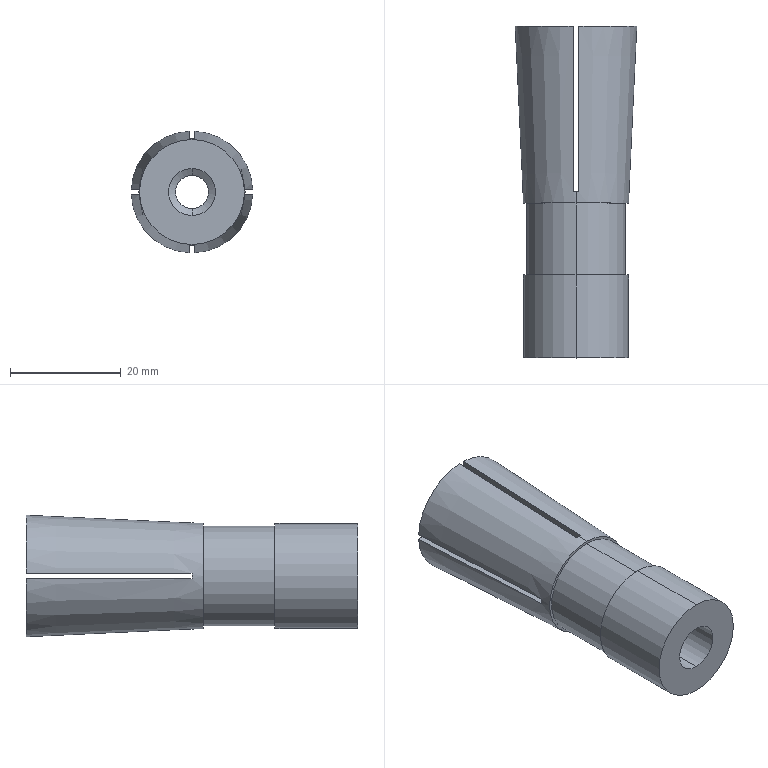Part | SolidWorks | features ICE 3, 3DProfileFeature 1, HoleWzd 1, Revolution 1 | 1 solid | 31 faces | box 21.977 x 60 x 21.977 mm | volume 14861 mm3 | plane 19 | cylinder 8 | cone 4 | commonest cylinder face diameters 6 x2 8.5 x2 18 x2 19 x2
STEP:
#1=CARTESIAN_POINT('',(0.,24.5,4.25));
#2=VERTEX_POINT('',#1);
#3=CARTESIAN_POINT('',(0.,24.5,-4.25));
#4=VERTEX_POINT('',#3);
#5=CARTESIAN_POINT('',(0.,24.5,0.));
#6=DIRECTION('',(0.,-1.,0.));
#7=DIRECTION('',(0.,0.,-1.));
#8=AXIS2_PLACEMENT_3D('',#5,#6,#7);
#9=CIRCLE('',#8,4.25);
#10=EDGE_CURVE('',#2,#4,#9,.T.);
#11=ORIENTED_EDGE('',*,*,#10,.F.);
#12=CARTESIAN_POINT('',(0.,0.,4.25));
#13=VERTEX_POINT('',#12);
#14=CARTESIAN_POINT('',(0.,0.,4.25));
#15=DIRECTION('',(0.,-1.,0.));
#16=VECTOR('',#15,1000.);
#17=LINE('',#14,#16);
#18=EDGE_CURVE('',#2,#13,#17,.T.);
#19=ORIENTED_EDGE('',*,*,#18,.T.);
#20=CARTESIAN_POINT('',(0.,0.,-4.25));
#21=VERTEX_POINT('',#20);
#22=CARTESIAN_POINT('',(0.,0.,0.));
#23=DIRECTION('',(0.,-1.,0.));
#24=DIRECTION('',(0.,0.,-1.));
#25=AXIS2_PLACEMENT_3D('',#22,#23,#24);
#26=CIRCLE('',#25,4.25);
#27=EDGE_CURVE('',#13,#21,#26,.T.);
#28=ORIENTED_EDGE('',*,*,#27,.T.);
#29=CARTESIAN_POINT('',(0.,0.,-4.25));
#30=DIRECTION('',(0.,-1.,0.));
#31=VECTOR('',#30,1000.);
#32=LINE('',#29,#31);
#33=EDGE_CURVE('',#4,#21,#32,.T.);
#34=ORIENTED_EDGE('',*,*,#33,.F.);
#35=EDGE_LOOP('',(#11,#19,#28,#34));
#36=FACE_OUTER_BOUND('',#35,.T.);
#37=CARTESIAN_POINT('',(0.,0.,0.));
#38=DIRECTION('',(0.,-1.,0.));
#39=DIRECTION('',(0.,0.,-1.));
#40=AXIS2_PLACEMENT_3D('',#37,#38,#39);
#41=CYLINDRICAL_SURFACE('',#40,4.25);
#42=ADVANCED_FACE('',(#36),#41,.F.);
#43=CARTESIAN_POINT('',(0.,25.251,3.));
#44=VERTEX_POINT('',#43);
#45=CARTESIAN_POINT('',(0.,25.251,-3.));
#46=VERTEX_POINT('',#45);
#47=CARTESIAN_POINT('',(0.,25.251,0.));
#48=DIRECTION('',(0.,-1.,0.));
#49=DIRECTION('',(0.,0.,-1.));
#50=AXIS2_PLACEMENT_3D('',#47,#48,#49);
#51=CIRCLE('',#50,3.);
#52=EDGE_CURVE('',#44,#46,#51,.T.);
#53=ORIENTED_EDGE('',*,*,#52,.F.);
#54=CARTESIAN_POINT('',(0.,24.5,4.25));
#55=DIRECTION('',(0.,-0.515,0.8572));
#56=VECTOR('',#55,1000.);
#57=LINE('',#54,#56);
#58=EDGE_CURVE('',#44,#2,#57,.T.);
#59=ORIENTED_EDGE('',*,*,#58,.T.);
#60=ORIENTED_EDGE('',*,*,#10,.T.);
#61=CARTESIAN_POINT('',(0.,24.5,-4.25));
#62=DIRECTION('',(0.,-0.515,-0.8572));
#63=VECTOR('',#62,1000.);
#64=LINE('',#61,#63);
#65=EDGE_CURVE('',#46,#4,#64,.T.);
#66=ORIENTED_EDGE('',*,*,#65,.F.);
#67=EDGE_LOOP('',(#53,#59,#60,#66));
#68=FACE_OUTER_BOUND('',#67,.T.);
#69=CARTESIAN_POINT('',(0.,24.5,0.));
#70=DIRECTION('',(0.,-1.,0.));
#71=DIRECTION('',(0.,0.,-1.));
#72=AXIS2_PLACEMENT_3D('',#69,#70,#71);
#73=CONICAL_SURFACE('',#72,4.25,1.03);
#74=ADVANCED_FACE('',(#68),#73,.F.);
#75=ORIENTED_EDGE('',*,*,#52,.T.);
#76=CARTESIAN_POINT('',(0.,30.,-3.));
#77=VERTEX_POINT('',#76);
#78=CARTESIAN_POINT('',(0.,0.,-3.));
#79=DIRECTION('',(0.,1.,0.));
#80=VECTOR('',#79,1000.);
#81=LINE('',#78,#80);
#82=EDGE_CURVE('',#46,#77,#81,.T.);
#83=ORIENTED_EDGE('',*,*,#82,.T.);
#84=CARTESIAN_POINT('',(-0.5,30.,-2.958));
#85=VERTEX_POINT('',#84);
#86=CARTESIAN_POINT('',(0.,30.,0.));
#87=DIRECTION('',(0.,1.,0.));
#88=DIRECTION('',(0.,0.,-1.));
#89=AXIS2_PLACEMENT_3D('',#86,#87,#88);
#90=CIRCLE('',#89,3.);
#91=EDGE_CURVE('',#77,#85,#90,.T.);
#92=ORIENTED_EDGE('',*,*,#91,.T.);
#93=CARTESIAN_POINT('',(-0.5,60.,-2.958));
#94=VERTEX_POINT('',#93);
#95=CARTESIAN_POINT('',(-0.5,0.,-2.958));
#96=DIRECTION('',(0.,1.,0.));
#97=VECTOR('',#96,1000.);
#98=LINE('',#95,#97);
#99=EDGE_CURVE('',#85,#94,#98,.T.);
#100=ORIENTED_EDGE('',*,*,#99,.T.);
#101=CARTESIAN_POINT('',(-2.958,60.,-0.5));
#102=VERTEX_POINT('',#101);
#103=CARTESIAN_POINT('',(0.,60.,0.));
#104=DIRECTION('',(0.,1.,0.));
#105=DIRECTION('',(0.,0.,1.));
#106=AXIS2_PLACEMENT_3D('',#103,#104,#105);
#107=CIRCLE('',#106,3.);
#108=EDGE_CURVE('',#94,#102,#107,.T.);
#109=ORIENTED_EDGE('',*,*,#108,.T.);
#110=CARTESIAN_POINT('',(-2.958,30.,-0.5));
#111=VERTEX_POINT('',#110);
#112=CARTESIAN_POINT('',(-2.958,0.,-0.5));
#113=DIRECTION('',(0.,-1.,0.));
#114=VECTOR('',#113,1000.);
#115=LINE('',#112,#114);
#116=EDGE_CURVE('',#102,#111,#115,.T.);
#117=ORIENTED_EDGE('',*,*,#116,.T.);
#118=CARTESIAN_POINT('',(-2.958,30.,0.5));
#119=VERTEX_POINT('',#118);
#120=CARTESIAN_POINT('',(0.,30.,0.));
#121=DIRECTION('',(0.,-1.,0.));
#122=DIRECTION('',(0.,0.,1.));
#123=AXIS2_PLACEMENT_3D('',#120,#121,#122);
#124=CIRCLE('',#123,3.);
#125=EDGE_CURVE('',#119,#111,#124,.T.);
#126=ORIENTED_EDGE('',*,*,#125,.F.);
#127=CARTESIAN_POINT('',(-2.958,60.,0.5));
#128=VERTEX_POINT('',#127);
#129=CARTESIAN_POINT('',(-2.958,0.,0.5));
#130=DIRECTION('',(0.,1.,0.));
#131=VECTOR('',#130,1000.);
#132=LINE('',#129,#131);
#133=EDGE_CURVE('',#119,#128,#132,.T.);
#134=ORIENTED_EDGE('',*,*,#133,.T.);
#135=CARTESIAN_POINT('',(-0.5,60.,2.958));
#136=VERTEX_POINT('',#135);
#137=CARTESIAN_POINT('',(0.,60.,0.));
#138=DIRECTION('',(0.,1.,0.));
#139=DIRECTION('',(0.,0.,1.));
#140=AXIS2_PLACEMENT_3D('',#137,#138,#139);
#141=CIRCLE('',#140,3.);
#142=EDGE_CURVE('',#128,#136,#141,.T.);
#143=ORIENTED_EDGE('',*,*,#142,.T.);
#144=CARTESIAN_POINT('',(-0.5,30.,2.958));
#145=VERTEX_POINT('',#144);
#146=CARTESIAN_POINT('',(-0.5,0.,2.958));
#147=DIRECTION('',(0.,-1.,0.));
#148=VECTOR('',#147,1000.);
#149=LINE('',#146,#148);
#150=EDGE_CURVE('',#136,#145,#149,.T.);
#151=ORIENTED_EDGE('',*,*,#150,.T.);
#152=CARTESIAN_POINT('',(0.,30.,3.));
#153=VERTEX_POINT('',#152);
#154=CARTESIAN_POINT('',(0.,30.,0.));
#155=DIRECTION('',(0.,1.,0.));
#156=DIRECTION('',(0.,0.,-1.));
#157=AXIS2_PLACEMENT_3D('',#154,#155,#156);
#158=CIRCLE('',#157,3.);
#159=EDGE_CURVE('',#145,#153,#158,.T.);
#160=ORIENTED_EDGE('',*,*,#159,.T.);
#161=CARTESIAN_POINT('',(0.,0.,3.));
#162=DIRECTION('',(0.,1.,0.));
#163=VECTOR('',#162,1000.);
#164=LINE('',#161,#163);
#165=EDGE_CURVE('',#44,#153,#164,.T.);
#166=ORIENTED_EDGE('',*,*,#165,.F.);
#167=EDGE_LOOP('',(#75,#83,#92,#100,#109,#117,#126,#134,#143,#151,#160,#166));
#168=FACE_OUTER_BOUND('',#167,.T.);
#169=CARTESIAN_POINT('',(0.,0.,0.));
#170=DIRECTION('',(0.,1.,0.));
#171=DIRECTION('',(0.,0.,1.));
#172=AXIS2_PLACEMENT_3D('',#169,#170,#171);
#173=CYLINDRICAL_SURFACE('',#172,3.);
#174=ADVANCED_FACE('',(#168),#173,.F.);
#175=CARTESIAN_POINT('',(0.,15.,-9.5));
#176=VERTEX_POINT('',#175);
#177=CARTESIAN_POINT('',(0.,15.,9.5));
#178=VERTEX_POINT('',#177);
#179=CARTESIAN_POINT('',(0.,15.,0.));
#180=DIRECTION('',(0.,-1.,0.));
#181=DIRECTION('',(0.,0.,-1.));
#182=AXIS2_PLACEMENT_3D('',#179,#180,#181);
#183=CIRCLE('',#182,9.5);
#184=EDGE_CURVE('',#176,#178,#183,.T.);
#185=ORIENTED_EDGE('',*,*,#184,.T.);
#186=CARTESIAN_POINT('',(0.,0.,9.5));
#187=VERTEX_POINT('',#186);
#188=CARTESIAN_POINT('',(0.,0.,9.5));
#189=DIRECTION('',(0.,-1.,0.));
#190=VECTOR('',#189,1000.);
#191=LINE('',#188,#190);
#192=EDGE_CURVE('',#178,#187,#191,.T.);
#193=ORIENTED_EDGE('',*,*,#192,.T.);
#194=CARTESIAN_POINT('',(0.,0.,-9.5));
#195=VERTEX_POINT('',#194);
#196=CARTESIAN_POINT('',(0.,0.,0.));
#197=DIRECTION('',(0.,-1.,0.));
#198=DIRECTION('',(0.,0.,-1.));
#199=AXIS2_PLACEMENT_3D('',#196,#197,#198);
#200=CIRCLE('',#199,9.5);
#201=EDGE_CURVE('',#195,#187,#200,.T.);
#202=ORIENTED_EDGE('',*,*,#201,.F.);
#203=CARTESIAN_POINT('',(0.,0.,-9.5));
#204=DIRECTION('',(0.,-1.,0.));
#205=VECTOR('',#204,1000.);
#206=LINE('',#203,#205);
#207=EDGE_CURVE('',#176,#195,#206,.T.);
#208=ORIENTED_EDGE('',*,*,#207,.F.);
#209=EDGE_LOOP('',(#185,#193,#202,#208));
#210=FACE_OUTER_BOUND('',#209,.T.);
#211=CARTESIAN_POINT('',(0.,0.,0.));
#212=DIRECTION('',(0.,-1.,0.));
#213=DIRECTION('',(0.,0.,-1.));
#214=AXIS2_PLACEMENT_3D('',#211,#212,#213);
#215=CYLINDRICAL_SURFACE('',#214,9.5);
#216=ADVANCED_FACE('',(#210),#215,.T.);
#217=CARTESIAN_POINT('',(0.,28.,-9.));
#218=VERTEX_POINT('',#217);
#219=CARTESIAN_POINT('',(0.,28.,9.));
#220=VERTEX_POINT('',#219);
#221=CARTESIAN_POINT('',(0.,28.,0.));
#222=DIRECTION('',(0.,-1.,0.));
#223=DIRECTION('',(0.,0.,-1.));
#224=AXIS2_PLACEMENT_3D('',#221,#222,#223);
#225=CIRCLE('',#224,9.);
#226=EDGE_CURVE('',#218,#220,#225,.T.);
#227=ORIENTED_EDGE('',*,*,#226,.T.);
#228=CARTESIAN_POINT('',(0.,15.,9.));
#229=VERTEX_POINT('',#228);
#230=CARTESIAN_POINT('',(0.,0.,9.));
#231=DIRECTION('',(0.,-1.,0.));
#232=VECTOR('',#231,1000.);
#233=LINE('',#230,#232);
#234=EDGE_CURVE('',#220,#229,#233,.T.);
#235=ORIENTED_EDGE('',*,*,#234,.T.);
#236=CARTESIAN_POINT('',(0.,15.,-9.));
#237=VERTEX_POINT('',#236);
#238=CARTESIAN_POINT('',(0.,15.,0.));
#239=DIRECTION('',(0.,-1.,0.));
#240=DIRECTION('',(0.,0.,-1.));
#241=AXIS2_PLACEMENT_3D('',#238,#239,#240);
#242=CIRCLE('',#241,9.);
#243=EDGE_CURVE('',#237,#229,#242,.T.);
#244=ORIENTED_EDGE('',*,*,#243,.F.);
#245=CARTESIAN_POINT('',(0.,0.,-9.));
#246=DIRECTION('',(0.,-1.,0.));
#247=VECTOR('',#246,1000.);
#248=LINE('',#245,#247);
#249=EDGE_CURVE('',#218,#237,#248,.T.);
#250=ORIENTED_EDGE('',*,*,#249,.F.);
#251=EDGE_LOOP('',(#227,#235,#244,#250));
#252=FACE_OUTER_BOUND('',#251,.T.);
#253=CARTESIAN_POINT('',(0.,0.,0.));
#254=DIRECTION('',(0.,-1.,0.));
#255=DIRECTION('',(0.,0.,-1.));
#256=AXIS2_PLACEMENT_3D('',#253,#254,#255);
#257=CYLINDRICAL_SURFACE('',#256,9.);
#258=ADVANCED_FACE('',(#252),#257,.T.);
#259=CARTESIAN_POINT('',(0.,28.,-9.5));
#260=VERTEX_POINT('',#259);
#261=CARTESIAN_POINT('',(0.,28.,9.5));
#262=VERTEX_POINT('',#261);
#263=CARTESIAN_POINT('',(0.,28.,0.));
#264=DIRECTION('',(0.,-1.,0.));
#265=DIRECTION('',(0.,0.,-1.));
#266=AXIS2_PLACEMENT_3D('',#263,#264,#265);
#267=CIRCLE('',#266,9.5);
#268=EDGE_CURVE('',#260,#262,#267,.T.);
#269=ORIENTED_EDGE('',*,*,#268,.F.);
#270=CARTESIAN_POINT('',(0.,30.,-9.594));
#271=VERTEX_POINT('',#270);
#272=CARTESIAN_POINT('',(0.,28.,-9.5));
#273=DIRECTION('',(0.,0.9989,-0.04682));
#274=VECTOR('',#273,1000.);
#275=LINE('',#272,#274);
#276=EDGE_CURVE('',#260,#271,#275,.T.);
#277=ORIENTED_EDGE('',*,*,#276,.T.);
#278=CARTESIAN_POINT('',(0.5,30.,-9.581));
#279=VERTEX_POINT('',#278);
#280=CARTESIAN_POINT('',(0.,30.,0.));
#281=DIRECTION('',(0.,1.,0.));
#282=DIRECTION('',(0.,0.,-1.));
#283=AXIS2_PLACEMENT_3D('',#280,#281,#282);
#284=CIRCLE('',#283,9.594);
#285=EDGE_CURVE('',#279,#271,#284,.T.);
#286=ORIENTED_EDGE('',*,*,#285,.F.);
#287=CARTESIAN_POINT('',(0.5,60.,-10.989));
#288=VERTEX_POINT('',#287);
#289=CARTESIAN_POINT('',(0.5,60.,-10.989));
#290=CARTESIAN_POINT('',(0.5,50.,-10.519));
#291=CARTESIAN_POINT('',(0.5,40.,-10.05));
#292=CARTESIAN_POINT('',(0.5,30.,-9.581));
#293=B_SPLINE_CURVE_WITH_KNOTS('',3,(#289,#290,#291,#292),.UNSPECIFIED.,.F.,.F.,(4,4),(0.03724,0.06728),.UNSPECIFIED.);
#294=EDGE_CURVE('',#288,#279,#293,.T.);
#295=ORIENTED_EDGE('',*,*,#294,.F.);
#296=CARTESIAN_POINT('',(10.989,60.,-0.5));
#297=VERTEX_POINT('',#296);
#298=CARTESIAN_POINT('',(0.,60.,0.));
#299=DIRECTION('',(0.,-1.,0.));
#300=DIRECTION('',(0.,0.,-1.));
#301=AXIS2_PLACEMENT_3D('',#298,#299,#300);
#302=CIRCLE('',#301,11.);
#303=EDGE_CURVE('',#288,#297,#302,.T.);
#304=ORIENTED_EDGE('',*,*,#303,.T.);
#305=CARTESIAN_POINT('',(9.581,30.,-0.5));
#306=VERTEX_POINT('',#305);
#307=CARTESIAN_POINT('',(9.581,30.,-0.5));
#308=CARTESIAN_POINT('',(10.05,40.,-0.5));
#309=CARTESIAN_POINT('',(10.519,50.,-0.5));
#310=CARTESIAN_POINT('',(10.989,60.,-0.5));
#311=B_SPLINE_CURVE_WITH_KNOTS('',3,(#307,#308,#309,#310),.UNSPECIFIED.,.F.,.F.,(4,4),(0.03724,0.06728),.UNSPECIFIED.);
#312=EDGE_CURVE('',#306,#297,#311,.T.);
#313=ORIENTED_EDGE('',*,*,#312,.F.);
#314=CARTESIAN_POINT('',(9.581,30.,0.5));
#315=VERTEX_POINT('',#314);
#316=CARTESIAN_POINT('',(0.,30.,0.));
#317=DIRECTION('',(0.,-1.,0.));
#318=DIRECTION('',(0.,0.,1.));
#319=AXIS2_PLACEMENT_3D('',#316,#317,#318);
#320=CIRCLE('',#319,9.594);
#321=EDGE_CURVE('',#306,#315,#320,.T.);
#322=ORIENTED_EDGE('',*,*,#321,.T.);
#323=CARTESIAN_POINT('',(10.989,60.,0.5));
#324=VERTEX_POINT('',#323);
#325=CARTESIAN_POINT('',(10.989,60.,0.5));
#326=CARTESIAN_POINT('',(10.519,50.,0.5));
#327=CARTESIAN_POINT('',(10.05,40.,0.5));
#328=CARTESIAN_POINT('',(9.581,30.,0.5));
#329=B_SPLINE_CURVE_WITH_KNOTS('',3,(#325,#326,#327,#328),.UNSPECIFIED.,.F.,.F.,(4,4),(0.03724,0.06728),.UNSPECIFIED.);
#330=EDGE_CURVE('',#324,#315,#329,.T.);
#331=ORIENTED_EDGE('',*,*,#330,.F.);
#332=CARTESIAN_POINT('',(0.5,60.,10.989));
#333=VERTEX_POINT('',#332);
#334=CARTESIAN_POINT('',(0.,60.,0.));
#335=DIRECTION('',(0.,-1.,0.));
#336=DIRECTION('',(0.,0.,-1.));
#337=AXIS2_PLACEMENT_3D('',#334,#335,#336);
#338=CIRCLE('',#337,11.);
#339=EDGE_CURVE('',#324,#333,#338,.T.);
#340=ORIENTED_EDGE('',*,*,#339,.T.);
#341=CARTESIAN_POINT('',(0.5,30.,9.581));
#342=VERTEX_POINT('',#341);
#343=CARTESIAN_POINT('',(0.5,30.,9.581));
#344=CARTESIAN_POINT('',(0.5,40.,10.05));
#345=CARTESIAN_POINT('',(0.5,50.,10.519));
#346=CARTESIAN_POINT('',(0.5,60.,10.989));
#347=B_SPLINE_CURVE_WITH_KNOTS('',3,(#343,#344,#345,#346),.UNSPECIFIED.,.F.,.F.,(4,4),(0.03724,0.06728),.UNSPECIFIED.);
#348=EDGE_CURVE('',#342,#333,#347,.T.);
#349=ORIENTED_EDGE('',*,*,#348,.F.);
#350=CARTESIAN_POINT('',(0.,30.,9.594));
#351=VERTEX_POINT('',#350);
#352=CARTESIAN_POINT('',(0.,30.,0.));
#353=DIRECTION('',(0.,1.,0.));
#354=DIRECTION('',(0.,0.,-1.));
#355=AXIS2_PLACEMENT_3D('',#352,#353,#354);
#356=CIRCLE('',#355,9.594);
#357=EDGE_CURVE('',#351,#342,#356,.T.);
#358=ORIENTED_EDGE('',*,*,#357,.F.);
#359=CARTESIAN_POINT('',(0.,28.,9.5));
#360=DIRECTION('',(0.,0.9989,0.04682));
#361=VECTOR('',#360,1000.);
#362=LINE('',#359,#361);
#363=EDGE_CURVE('',#262,#351,#362,.T.);
#364=ORIENTED_EDGE('',*,*,#363,.F.);
#365=EDGE_LOOP('',(#269,#277,#286,#295,#304,#313,#322,#331,#340,#349,#358,#364));
#366=FACE_OUTER_BOUND('',#365,.T.);
#367=CARTESIAN_POINT('',(0.,28.,0.));
#368=DIRECTION('',(0.,1.,0.));
#369=DIRECTION('',(0.,0.,1.));
#370=AXIS2_PLACEMENT_3D('',#367,#368,#369);
#371=CONICAL_SURFACE('',#370,9.5,0.04684);
#372=ADVANCED_FACE('',(#366),#371,.T.);
#373=CARTESIAN_POINT('',(-0.5,60.,10.989));
#374=VERTEX_POINT('',#373);
#375=CARTESIAN_POINT('',(-0.5,60.,-25.));
#376=DIRECTION('',(0.,0.,1.));
#377=VECTOR('',#376,1000.);
#378=LINE('',#375,#377);
#379=EDGE_CURVE('',#136,#374,#378,.T.);
#380=ORIENTED_EDGE('',*,*,#379,.F.);
#381=ORIENTED_EDGE('',*,*,#142,.F.);
#382=CARTESIAN_POINT('',(-10.989,60.,0.5));
#383=VERTEX_POINT('',#382);
#384=CARTESIAN_POINT('',(-25.,60.,0.5));
#385=DIRECTION('',(1.,0.,0.));
#386=VECTOR('',#385,1000.);
#387=LINE('',#384,#386);
#388=EDGE_CURVE('',#383,#128,#387,.T.);
#389=ORIENTED_EDGE('',*,*,#388,.F.);
#390=CARTESIAN_POINT('',(0.,60.,0.));
#391=DIRECTION('',(0.,-1.,0.));
#392=DIRECTION('',(0.,0.,-1.));
#393=AXIS2_PLACEMENT_3D('',#390,#391,#392);
#394=CIRCLE('',#393,11.);
#395=EDGE_CURVE('',#374,#383,#394,.T.);
#396=ORIENTED_EDGE('',*,*,#395,.F.);
#397=EDGE_LOOP('',(#380,#381,#389,#396));
#398=FACE_OUTER_BOUND('',#397,.T.);
#399=CARTESIAN_POINT('',(0.,60.,0.));
#400=DIRECTION('',(0.,1.,0.));
#401=DIRECTION('',(0.,0.,1.));
#402=AXIS2_PLACEMENT_3D('',#399,#400,#401);
#403=PLANE('',#402);
#404=ADVANCED_FACE('',(#398),#403,.T.);
#405=CARTESIAN_POINT('',(-0.5,60.,-10.989));
#406=VERTEX_POINT('',#405);
#407=CARTESIAN_POINT('',(-0.5,60.,-25.));
#408=DIRECTION('',(0.,0.,1.));
#409=VECTOR('',#408,1000.);
#410=LINE('',#407,#409);
#411=EDGE_CURVE('',#406,#94,#410,.T.);
#412=ORIENTED_EDGE('',*,*,#411,.F.);
#413=CARTESIAN_POINT('',(-10.989,60.,-0.5));
#414=VERTEX_POINT('',#413);
#415=CARTESIAN_POINT('',(0.,60.,0.));
#416=DIRECTION('',(0.,-1.,0.));
#417=DIRECTION('',(0.,0.,-1.));
#418=AXIS2_PLACEMENT_3D('',#415,#416,#417);
#419=CIRCLE('',#418,11.);
#420=EDGE_CURVE('',#414,#406,#419,.T.);
#421=ORIENTED_EDGE('',*,*,#420,.F.);
#422=CARTESIAN_POINT('',(-25.,60.,-0.5));
#423=DIRECTION('',(-1.,0.,0.));
#424=VECTOR('',#423,1000.);
#425=LINE('',#422,#424);
#426=EDGE_CURVE('',#102,#414,#425,.T.);
#427=ORIENTED_EDGE('',*,*,#426,.F.);
#428=ORIENTED_EDGE('',*,*,#108,.F.);
#429=EDGE_LOOP('',(#412,#421,#427,#428));
#430=FACE_OUTER_BOUND('',#429,.T.);
#431=CARTESIAN_POINT('',(0.,60.,0.));
#432=DIRECTION('',(0.,1.,0.));
#433=DIRECTION('',(0.,0.,1.));
#434=AXIS2_PLACEMENT_3D('',#431,#432,#433);
#435=PLANE('',#434);
#436=ADVANCED_FACE('',(#430),#435,.T.);
#437=CARTESIAN_POINT('',(0.5,60.,2.958));
#438=VERTEX_POINT('',#437);
#439=CARTESIAN_POINT('',(0.5,60.,-25.));
#440=DIRECTION('',(0.,0.,-1.));
#441=VECTOR('',#440,1000.);
#442=LINE('',#439,#441);
#443=EDGE_CURVE('',#333,#438,#442,.T.);
#444=ORIENTED_EDGE('',*,*,#443,.F.);
#445=ORIENTED_EDGE('',*,*,#339,.F.);
#446=CARTESIAN_POINT('',(2.958,60.,0.5));
#447=VERTEX_POINT('',#446);
#448=CARTESIAN_POINT('',(-25.,60.,0.5));
#449=DIRECTION('',(1.,0.,0.));
#450=VECTOR('',#449,1000.);
#451=LINE('',#448,#450);
#452=EDGE_CURVE('',#447,#324,#451,.T.);
#453=ORIENTED_EDGE('',*,*,#452,.F.);
#454=CARTESIAN_POINT('',(0.,60.,0.));
#455=DIRECTION('',(0.,1.,0.));
#456=DIRECTION('',(0.,0.,1.));
#457=AXIS2_PLACEMENT_3D('',#454,#455,#456);
#458=CIRCLE('',#457,3.);
#459=EDGE_CURVE('',#438,#447,#458,.T.);
#460=ORIENTED_EDGE('',*,*,#459,.F.);
#461=EDGE_LOOP('',(#444,#445,#453,#460));
#462=FACE_OUTER_BOUND('',#461,.T.);
#463=CARTESIAN_POINT('',(0.,60.,0.));
#464=DIRECTION('',(0.,1.,0.));
#465=DIRECTION('',(0.,0.,1.));
#466=AXIS2_PLACEMENT_3D('',#463,#464,#465);
#467=PLANE('',#466);
#468=ADVANCED_FACE('',(#462),#467,.T.);
#469=CARTESIAN_POINT('',(0.5,60.,-2.958));
#470=VERTEX_POINT('',#469);
#471=CARTESIAN_POINT('',(0.5,60.,-25.));
#472=DIRECTION('',(0.,0.,-1.));
#473=VECTOR('',#472,1000.);
#474=LINE('',#471,#473);
#475=EDGE_CURVE('',#470,#288,#474,.T.);
#476=ORIENTED_EDGE('',*,*,#475,.F.);
#477=CARTESIAN_POINT('',(2.958,60.,-0.5));
#478=VERTEX_POINT('',#477);
#479=CARTESIAN_POINT('',(0.,60.,0.));
#480=DIRECTION('',(0.,1.,0.));
#481=DIRECTION('',(0.,0.,1.));
#482=AXIS2_PLACEMENT_3D('',#479,#480,#481);
#483=CIRCLE('',#482,3.);
#484=EDGE_CURVE('',#478,#470,#483,.T.);
#485=ORIENTED_EDGE('',*,*,#484,.F.);
#486=CARTESIAN_POINT('',(-25.,60.,-0.5));
#487=DIRECTION('',(-1.,0.,0.));
#488=VECTOR('',#487,1000.);
#489=LINE('',#486,#488);
#490=EDGE_CURVE('',#297,#478,#489,.T.);
#491=ORIENTED_EDGE('',*,*,#490,.F.);
#492=ORIENTED_EDGE('',*,*,#303,.F.);
#493=EDGE_LOOP('',(#476,#485,#491,#492));
#494=FACE_OUTER_BOUND('',#493,.T.);
#495=CARTESIAN_POINT('',(0.,60.,0.));
#496=DIRECTION('',(0.,1.,0.));
#497=DIRECTION('',(0.,0.,1.));
#498=AXIS2_PLACEMENT_3D('',#495,#496,#497);
#499=PLANE('',#498);
#500=ADVANCED_FACE('',(#494),#499,.T.);
#501=ORIENTED_EDGE('',*,*,#276,.F.);
#502=CARTESIAN_POINT('',(0.,28.,0.));
#503=DIRECTION('',(0.,-1.,0.));
#504=DIRECTION('',(0.,0.,-1.));
#505=AXIS2_PLACEMENT_3D('',#502,#503,#504);
#506=CIRCLE('',#505,9.5);
#507=EDGE_CURVE('',#262,#260,#506,.T.);
#508=ORIENTED_EDGE('',*,*,#507,.F.);
#509=ORIENTED_EDGE('',*,*,#363,.T.);
#510=CARTESIAN_POINT('',(-0.5,30.,9.581));
#511=VERTEX_POINT('',#510);
#512=CARTESIAN_POINT('',(0.,30.,0.));
#513=DIRECTION('',(0.,1.,0.));
#514=DIRECTION('',(0.,0.,-1.));
#515=AXIS2_PLACEMENT_3D('',#512,#513,#514);
#516=CIRCLE('',#515,9.594);
#517=EDGE_CURVE('',#511,#351,#516,.T.);
#518=ORIENTED_EDGE('',*,*,#517,.F.);
#519=CARTESIAN_POINT('',(-0.5,60.,10.989));
#520=CARTESIAN_POINT('',(-0.5,50.,10.519));
#521=CARTESIAN_POINT('',(-0.5,40.,10.05));
#522=CARTESIAN_POINT('',(-0.5,30.,9.581));
#523=B_SPLINE_CURVE_WITH_KNOTS('',3,(#519,#520,#521,#522),.UNSPECIFIED.,.F.,.F.,(4,4),(0.03724,0.06728),.UNSPECIFIED.);
#524=EDGE_CURVE('',#374,#511,#523,.T.);
#525=ORIENTED_EDGE('',*,*,#524,.F.);
#526=ORIENTED_EDGE('',*,*,#395,.T.);
#527=CARTESIAN_POINT('',(-9.581,30.,0.5));
#528=VERTEX_POINT('',#527);
#529=CARTESIAN_POINT('',(-9.581,30.,0.5));
#530=CARTESIAN_POINT('',(-10.05,40.,0.5));
#531=CARTESIAN_POINT('',(-10.519,50.,0.5));
#532=CARTESIAN_POINT('',(-10.989,60.,0.5));
#533=B_SPLINE_CURVE_WITH_KNOTS('',3,(#529,#530,#531,#532),.UNSPECIFIED.,.F.,.F.,(4,4),(0.03724,0.06728),.UNSPECIFIED.);
#534=EDGE_CURVE('',#528,#383,#533,.T.);
#535=ORIENTED_EDGE('',*,*,#534,.F.);
#536=CARTESIAN_POINT('',(-9.581,30.,-0.5));
#537=VERTEX_POINT('',#536);
#538=CARTESIAN_POINT('',(0.,30.,0.));
#539=DIRECTION('',(0.,-1.,0.));
#540=DIRECTION('',(0.,0.,1.));
#541=AXIS2_PLACEMENT_3D('',#538,#539,#540);
#542=CIRCLE('',#541,9.594);
#543=EDGE_CURVE('',#528,#537,#542,.T.);
#544=ORIENTED_EDGE('',*,*,#543,.T.);
#545=CARTESIAN_POINT('',(-10.989,60.,-0.5));
#546=CARTESIAN_POINT('',(-10.519,50.,-0.5));
#547=CARTESIAN_POINT('',(-10.05,40.,-0.5));
#548=CARTESIAN_POINT('',(-9.581,30.,-0.5));
#549=B_SPLINE_CURVE_WITH_KNOTS('',3,(#545,#546,#547,#548),.UNSPECIFIED.,.F.,.F.,(4,4),(0.03724,0.06728),.UNSPECIFIED.);
#550=EDGE_CURVE('',#414,#537,#549,.T.);
#551=ORIENTED_EDGE('',*,*,#550,.F.);
#552=ORIENTED_EDGE('',*,*,#420,.T.);
#553=CARTESIAN_POINT('',(-0.5,30.,-9.581));
#554=VERTEX_POINT('',#553);
#555=CARTESIAN_POINT('',(-0.5,30.,-9.581));
#556=CARTESIAN_POINT('',(-0.5,40.,-10.05));
#557=CARTESIAN_POINT('',(-0.5,50.,-10.519));
#558=CARTESIAN_POINT('',(-0.5,60.,-10.989));
#559=B_SPLINE_CURVE_WITH_KNOTS('',3,(#555,#556,#557,#558),.UNSPECIFIED.,.F.,.F.,(4,4),(0.03724,0.06728),.UNSPECIFIED.);
#560=EDGE_CURVE('',#554,#406,#559,.T.);
#561=ORIENTED_EDGE('',*,*,#560,.F.);
#562=CARTESIAN_POINT('',(0.,30.,0.));
#563=DIRECTION('',(0.,1.,0.));
#564=DIRECTION('',(0.,0.,-1.));
#565=AXIS2_PLACEMENT_3D('',#562,#563,#564);
#566=CIRCLE('',#565,9.594);
#567=EDGE_CURVE('',#271,#554,#566,.T.);
#568=ORIENTED_EDGE('',*,*,#567,.F.);
#569=EDGE_LOOP('',(#501,#508,#509,#518,#525,#526,#535,#544,#551,#552,#561,#568));
#570=FACE_OUTER_BOUND('',#569,.T.);
#571=CARTESIAN_POINT('',(0.,28.,0.));
#572=DIRECTION('',(0.,1.,0.));
#573=DIRECTION('',(0.,0.,1.));
#574=AXIS2_PLACEMENT_3D('',#571,#572,#573);
#575=CONICAL_SURFACE('',#574,9.5,0.04684);
#576=ADVANCED_FACE('',(#570),#575,.T.);
#577=ORIENTED_EDGE('',*,*,#507,.T.);
#578=ORIENTED_EDGE('',*,*,#268,.T.);
#579=EDGE_LOOP('',(#577,#578));
#580=FACE_OUTER_BOUND('',#579,.T.);
#581=ORIENTED_EDGE('',*,*,#226,.F.);
#582=CARTESIAN_POINT('',(0.,28.,0.));
#583=DIRECTION('',(0.,-1.,0.));
#584=DIRECTION('',(0.,0.,-1.));
#585=AXIS2_PLACEMENT_3D('',#582,#583,#584);
#586=CIRCLE('',#585,9.);
#587=EDGE_CURVE('',#220,#218,#586,.T.);
#588=ORIENTED_EDGE('',*,*,#587,.F.);
#589=EDGE_LOOP('',(#581,#588));
#590=FACE_BOUND('',#589,.T.);
#591=CARTESIAN_POINT('',(9.5,28.,0.));
#592=DIRECTION('',(0.,-1.,0.));
#593=DIRECTION('',(0.,0.,-1.));
#594=AXIS2_PLACEMENT_3D('',#591,#592,#593);
#595=PLANE('',#594);
#596=ADVANCED_FACE('',(#580,#590),#595,.T.);
#597=ORIENTED_EDGE('',*,*,#234,.F.);
#598=ORIENTED_EDGE('',*,*,#587,.T.);
#599=ORIENTED_EDGE('',*,*,#249,.T.);
#600=CARTESIAN_POINT('',(0.,15.,0.));
#601=DIRECTION('',(0.,-1.,0.));
#602=DIRECTION('',(0.,0.,-1.));
#603=AXIS2_PLACEMENT_3D('',#600,#601,#602);
#604=CIRCLE('',#603,9.);
#605=EDGE_CURVE('',#229,#237,#604,.T.);
#606=ORIENTED_EDGE('',*,*,#605,.F.);
#607=EDGE_LOOP('',(#597,#598,#599,#606));
#608=FACE_OUTER_BOUND('',#607,.T.);
#609=CARTESIAN_POINT('',(0.,0.,0.));
#610=DIRECTION('',(0.,-1.,0.));
#611=DIRECTION('',(0.,0.,-1.));
#612=AXIS2_PLACEMENT_3D('',#609,#610,#611);
#613=CYLINDRICAL_SURFACE('',#612,9.);
#614=ADVANCED_FACE('',(#608),#613,.T.);
#615=ORIENTED_EDGE('',*,*,#243,.T.);
#616=ORIENTED_EDGE('',*,*,#605,.T.);
#617=EDGE_LOOP('',(#615,#616));
#618=FACE_BOUND('',#617,.T.);
#619=ORIENTED_EDGE('',*,*,#184,.F.);
#620=CARTESIAN_POINT('',(0.,15.,0.));
#621=DIRECTION('',(0.,-1.,0.));
#622=DIRECTION('',(0.,0.,-1.));
#623=AXIS2_PLACEMENT_3D('',#620,#621,#622);
#624=CIRCLE('',#623,9.5);
#625=EDGE_CURVE('',#178,#176,#624,.T.);
#626=ORIENTED_EDGE('',*,*,#625,.F.);
#627=EDGE_LOOP('',(#619,#626));
#628=FACE_OUTER_BOUND('',#627,.T.);
#629=CARTESIAN_POINT('',(9.,15.,0.));
#630=DIRECTION('',(0.,1.,0.));
#631=DIRECTION('',(0.,0.,1.));
#632=AXIS2_PLACEMENT_3D('',#629,#630,#631);
#633=PLANE('',#632);
#634=ADVANCED_FACE('',(#618,#628),#633,.T.);
#635=ORIENTED_EDGE('',*,*,#192,.F.);
#636=ORIENTED_EDGE('',*,*,#625,.T.);
#637=ORIENTED_EDGE('',*,*,#207,.T.);
#638=CARTESIAN_POINT('',(0.,0.,0.));
#639=DIRECTION('',(0.,-1.,0.));
#640=DIRECTION('',(0.,0.,-1.));
#641=AXIS2_PLACEMENT_3D('',#638,#639,#640);
#642=CIRCLE('',#641,9.5);
#643=EDGE_CURVE('',#187,#195,#642,.T.);
#644=ORIENTED_EDGE('',*,*,#643,.F.);
#645=EDGE_LOOP('',(#635,#636,#637,#644));
#646=FACE_OUTER_BOUND('',#645,.T.);
#647=CARTESIAN_POINT('',(0.,0.,0.));
#648=DIRECTION('',(0.,-1.,0.));
#649=DIRECTION('',(0.,0.,-1.));
#650=AXIS2_PLACEMENT_3D('',#647,#648,#649);
#651=CYLINDRICAL_SURFACE('',#650,9.5);
#652=ADVANCED_FACE('',(#646),#651,.T.);
#653=CARTESIAN_POINT('',(0.,0.,0.));
#654=DIRECTION('',(0.,-1.,0.));
#655=DIRECTION('',(0.,0.,-1.));
#656=AXIS2_PLACEMENT_3D('',#653,#654,#655);
#657=CIRCLE('',#656,4.25);
#658=EDGE_CURVE('',#21,#13,#657,.T.);
#659=ORIENTED_EDGE('',*,*,#658,.F.);
#660=ORIENTED_EDGE('',*,*,#27,.F.);
#661=EDGE_LOOP('',(#659,#660));
#662=FACE_BOUND('',#661,.T.);
#663=ORIENTED_EDGE('',*,*,#201,.T.);
#664=ORIENTED_EDGE('',*,*,#643,.T.);
#665=EDGE_LOOP('',(#663,#664));
#666=FACE_OUTER_BOUND('',#665,.T.);
#667=CARTESIAN_POINT('',(9.5,0.,0.));
#668=DIRECTION('',(0.,-1.,0.));
#669=DIRECTION('',(0.,0.,-1.));
#670=AXIS2_PLACEMENT_3D('',#667,#668,#669);
#671=PLANE('',#670);
#672=ADVANCED_FACE('',(#662,#666),#671,.T.);
#673=ORIENTED_EDGE('',*,*,#82,.F.);
#674=CARTESIAN_POINT('',(0.,25.251,0.));
#675=DIRECTION('',(0.,-1.,0.));
#676=DIRECTION('',(0.,0.,-1.));
#677=AXIS2_PLACEMENT_3D('',#674,#675,#676);
#678=CIRCLE('',#677,3.);
#679=EDGE_CURVE('',#46,#44,#678,.T.);
#680=ORIENTED_EDGE('',*,*,#679,.T.);
#681=ORIENTED_EDGE('',*,*,#165,.T.);
#682=CARTESIAN_POINT('',(0.5,30.,2.958));
#683=VERTEX_POINT('',#682);
#684=CARTESIAN_POINT('',(0.,30.,0.));
#685=DIRECTION('',(0.,1.,0.));
#686=DIRECTION('',(0.,0.,-1.));
#687=AXIS2_PLACEMENT_3D('',#684,#685,#686);
#688=CIRCLE('',#687,3.);
#689=EDGE_CURVE('',#153,#683,#688,.T.);
#690=ORIENTED_EDGE('',*,*,#689,.T.);
#691=CARTESIAN_POINT('',(0.5,0.,2.958));
#692=DIRECTION('',(0.,1.,0.));
#693=VECTOR('',#692,1000.);
#694=LINE('',#691,#693);
#695=EDGE_CURVE('',#683,#438,#694,.T.);
#696=ORIENTED_EDGE('',*,*,#695,.T.);
#697=ORIENTED_EDGE('',*,*,#459,.T.);
#698=CARTESIAN_POINT('',(2.958,30.,0.5));
#699=VERTEX_POINT('',#698);
#700=CARTESIAN_POINT('',(2.958,0.,0.5));
#701=DIRECTION('',(0.,-1.,0.));
#702=VECTOR('',#701,1000.);
#703=LINE('',#700,#702);
#704=EDGE_CURVE('',#447,#699,#703,.T.);
#705=ORIENTED_EDGE('',*,*,#704,.T.);
#706=CARTESIAN_POINT('',(2.958,30.,-0.5));
#707=VERTEX_POINT('',#706);
#708=CARTESIAN_POINT('',(0.,30.,0.));
#709=DIRECTION('',(0.,-1.,0.));
#710=DIRECTION('',(0.,0.,1.));
#711=AXIS2_PLACEMENT_3D('',#708,#709,#710);
#712=CIRCLE('',#711,3.);
#713=EDGE_CURVE('',#707,#699,#712,.T.);
#714=ORIENTED_EDGE('',*,*,#713,.F.);
#715=CARTESIAN_POINT('',(2.958,0.,-0.5));
#716=DIRECTION('',(0.,1.,0.));
#717=VECTOR('',#716,1000.);
#718=LINE('',#715,#717);
#719=EDGE_CURVE('',#707,#478,#718,.T.);
#720=ORIENTED_EDGE('',*,*,#719,.T.);
#721=ORIENTED_EDGE('',*,*,#484,.T.);
#722=CARTESIAN_POINT('',(0.5,30.,-2.958));
#723=VERTEX_POINT('',#722);
#724=CARTESIAN_POINT('',(0.5,0.,-2.958));
#725=DIRECTION('',(0.,-1.,0.));
#726=VECTOR('',#725,1000.);
#727=LINE('',#724,#726);
#728=EDGE_CURVE('',#470,#723,#727,.T.);
#729=ORIENTED_EDGE('',*,*,#728,.T.);
#730=CARTESIAN_POINT('',(0.,30.,0.));
#731=DIRECTION('',(0.,1.,0.));
#732=DIRECTION('',(0.,0.,-1.));
#733=AXIS2_PLACEMENT_3D('',#730,#731,#732);
#734=CIRCLE('',#733,3.);
#735=EDGE_CURVE('',#723,#77,#734,.T.);
#736=ORIENTED_EDGE('',*,*,#735,.T.);
#737=EDGE_LOOP('',(#673,#680,#681,#690,#696,#697,#705,#714,#720,#721,#729,#736));
#738=FACE_OUTER_BOUND('',#737,.T.);
#739=CARTESIAN_POINT('',(0.,0.,0.));
#740=DIRECTION('',(0.,1.,0.));
#741=DIRECTION('',(0.,0.,1.));
#742=AXIS2_PLACEMENT_3D('',#739,#740,#741);
#743=CYLINDRICAL_SURFACE('',#742,3.);
#744=ADVANCED_FACE('',(#738),#743,.F.);
#745=ORIENTED_EDGE('',*,*,#58,.F.);
#746=ORIENTED_EDGE('',*,*,#679,.F.);
#747=ORIENTED_EDGE('',*,*,#65,.T.);
#748=CARTESIAN_POINT('',(0.,24.5,0.));
#749=DIRECTION('',(0.,-1.,0.));
#750=DIRECTION('',(0.,0.,-1.));
#751=AXIS2_PLACEMENT_3D('',#748,#749,#750);
#752=CIRCLE('',#751,4.25);
#753=EDGE_CURVE('',#4,#2,#752,.T.);
#754=ORIENTED_EDGE('',*,*,#753,.T.);
#755=EDGE_LOOP('',(#745,#746,#747,#754));
#756=FACE_OUTER_BOUND('',#755,.T.);
#757=CARTESIAN_POINT('',(0.,24.5,0.));
#758=DIRECTION('',(0.,-1.,0.));
#759=DIRECTION('',(0.,0.,-1.));
#760=AXIS2_PLACEMENT_3D('',#757,#758,#759);
#761=CONICAL_SURFACE('',#760,4.25,1.03);
#762=ADVANCED_FACE('',(#756),#761,.F.);
#763=ORIENTED_EDGE('',*,*,#18,.F.);
#764=ORIENTED_EDGE('',*,*,#753,.F.);
#765=ORIENTED_EDGE('',*,*,#33,.T.);
#766=ORIENTED_EDGE('',*,*,#658,.T.);
#767=EDGE_LOOP('',(#763,#764,#765,#766));
#768=FACE_OUTER_BOUND('',#767,.T.);
#769=CARTESIAN_POINT('',(0.,0.,0.));
#770=DIRECTION('',(0.,-1.,0.));
#771=DIRECTION('',(0.,0.,-1.));
#772=AXIS2_PLACEMENT_3D('',#769,#770,#771);
#773=CYLINDRICAL_SURFACE('',#772,4.25);
#774=ADVANCED_FACE('',(#768),#773,.F.);
#775=CARTESIAN_POINT('',(-25.,30.,-0.5));
#776=DIRECTION('',(-1.,0.,0.));
#777=VECTOR('',#776,1000.);
#778=LINE('',#775,#777);
#779=EDGE_CURVE('',#306,#707,#778,.T.);
#780=ORIENTED_EDGE('',*,*,#779,.T.);
#781=ORIENTED_EDGE('',*,*,#713,.T.);
#782=CARTESIAN_POINT('',(-25.,30.,0.5));
#783=DIRECTION('',(1.,0.,0.));
#784=VECTOR('',#783,1000.);
#785=LINE('',#782,#784);
#786=EDGE_CURVE('',#699,#315,#785,.T.);
#787=ORIENTED_EDGE('',*,*,#786,.T.);
#788=ORIENTED_EDGE('',*,*,#321,.F.);
#789=EDGE_LOOP('',(#780,#781,#787,#788));
#790=FACE_OUTER_BOUND('',#789,.T.);
#791=CARTESIAN_POINT('',(0.,30.,0.));
#792=DIRECTION('',(0.,1.,0.));
#793=DIRECTION('',(0.,0.,1.));
#794=AXIS2_PLACEMENT_3D('',#791,#792,#793);
#795=PLANE('',#794);
#796=ADVANCED_FACE('',(#790),#795,.T.);
#797=ORIENTED_EDGE('',*,*,#312,.T.);
#798=ORIENTED_EDGE('',*,*,#490,.T.);
#799=ORIENTED_EDGE('',*,*,#719,.F.);
#800=ORIENTED_EDGE('',*,*,#779,.F.);
#801=EDGE_LOOP('',(#797,#798,#799,#800));
#802=FACE_OUTER_BOUND('',#801,.T.);
#803=CARTESIAN_POINT('',(-25.,30.,-0.5));
#804=DIRECTION('',(0.,0.,-1.));
#805=DIRECTION('',(-1.,0.,0.));
#806=AXIS2_PLACEMENT_3D('',#803,#804,#805);
#807=PLANE('',#806);
#808=ADVANCED_FACE('',(#802),#807,.F.);
#809=ORIENTED_EDGE('',*,*,#330,.T.);
#810=ORIENTED_EDGE('',*,*,#786,.F.);
#811=ORIENTED_EDGE('',*,*,#704,.F.);
#812=ORIENTED_EDGE('',*,*,#452,.T.);
#813=EDGE_LOOP('',(#809,#810,#811,#812));
#814=FACE_OUTER_BOUND('',#813,.T.);
#815=CARTESIAN_POINT('',(-25.,30.,0.5));
#816=DIRECTION('',(0.,0.,1.));
#817=DIRECTION('',(1.,0.,0.));
#818=AXIS2_PLACEMENT_3D('',#815,#816,#817);
#819=PLANE('',#818);
#820=ADVANCED_FACE('',(#814),#819,.F.);
#821=ORIENTED_EDGE('',*,*,#534,.T.);
#822=ORIENTED_EDGE('',*,*,#388,.T.);
#823=ORIENTED_EDGE('',*,*,#133,.F.);
#824=CARTESIAN_POINT('',(-25.,30.,0.5));
#825=DIRECTION('',(1.,0.,0.));
#826=VECTOR('',#825,1000.);
#827=LINE('',#824,#826);
#828=EDGE_CURVE('',#528,#119,#827,.T.);
#829=ORIENTED_EDGE('',*,*,#828,.F.);
#830=EDGE_LOOP('',(#821,#822,#823,#829));
#831=FACE_OUTER_BOUND('',#830,.T.);
#832=CARTESIAN_POINT('',(-25.,30.,0.5));
#833=DIRECTION('',(0.,0.,1.));
#834=DIRECTION('',(1.,0.,0.));
#835=AXIS2_PLACEMENT_3D('',#832,#833,#834);
#836=PLANE('',#835);
#837=ADVANCED_FACE('',(#831),#836,.F.);
#838=ORIENTED_EDGE('',*,*,#550,.T.);
#839=CARTESIAN_POINT('',(-25.,30.,-0.5));
#840=DIRECTION('',(-1.,0.,0.));
#841=VECTOR('',#840,1000.);
#842=LINE('',#839,#841);
#843=EDGE_CURVE('',#111,#537,#842,.T.);
#844=ORIENTED_EDGE('',*,*,#843,.F.);
#845=ORIENTED_EDGE('',*,*,#116,.F.);
#846=ORIENTED_EDGE('',*,*,#426,.T.);
#847=EDGE_LOOP('',(#838,#844,#845,#846));
#848=FACE_OUTER_BOUND('',#847,.T.);
#849=CARTESIAN_POINT('',(-25.,30.,-0.5));
#850=DIRECTION('',(0.,0.,-1.));
#851=DIRECTION('',(-1.,0.,0.));
#852=AXIS2_PLACEMENT_3D('',#849,#850,#851);
#853=PLANE('',#852);
#854=ADVANCED_FACE('',(#848),#853,.F.);
#855=ORIENTED_EDGE('',*,*,#828,.T.);
#856=ORIENTED_EDGE('',*,*,#125,.T.);
#857=ORIENTED_EDGE('',*,*,#843,.T.);
#858=ORIENTED_EDGE('',*,*,#543,.F.);
#859=EDGE_LOOP('',(#855,#856,#857,#858));
#860=FACE_OUTER_BOUND('',#859,.T.);
#861=CARTESIAN_POINT('',(0.,30.,0.));
#862=DIRECTION('',(0.,1.,0.));
#863=DIRECTION('',(0.,0.,1.));
#864=AXIS2_PLACEMENT_3D('',#861,#862,#863);
#865=PLANE('',#864);
#866=ADVANCED_FACE('',(#860),#865,.T.);
#867=ORIENTED_EDGE('',*,*,#285,.T.);
#868=ORIENTED_EDGE('',*,*,#567,.T.);
#869=CARTESIAN_POINT('',(-0.5,30.,-25.));
#870=DIRECTION('',(0.,0.,1.));
#871=VECTOR('',#870,1000.);
#872=LINE('',#869,#871);
#873=EDGE_CURVE('',#554,#85,#872,.T.);
#874=ORIENTED_EDGE('',*,*,#873,.T.);
#875=ORIENTED_EDGE('',*,*,#91,.F.);
#876=ORIENTED_EDGE('',*,*,#735,.F.);
#877=CARTESIAN_POINT('',(0.5,30.,-25.));
#878=DIRECTION('',(0.,0.,-1.));
#879=VECTOR('',#878,1000.);
#880=LINE('',#877,#879);
#881=EDGE_CURVE('',#723,#279,#880,.T.);
#882=ORIENTED_EDGE('',*,*,#881,.T.);
#883=EDGE_LOOP('',(#867,#868,#874,#875,#876,#882));
#884=FACE_OUTER_BOUND('',#883,.T.);
#885=CARTESIAN_POINT('',(0.,30.,0.));
#886=DIRECTION('',(0.,-1.,0.));
#887=DIRECTION('',(0.,0.,-1.));
#888=AXIS2_PLACEMENT_3D('',#885,#886,#887);
#889=PLANE('',#888);
#890=ADVANCED_FACE('',(#884),#889,.F.);
#891=ORIENTED_EDGE('',*,*,#294,.T.);
#892=ORIENTED_EDGE('',*,*,#881,.F.);
#893=ORIENTED_EDGE('',*,*,#728,.F.);
#894=ORIENTED_EDGE('',*,*,#475,.T.);
#895=EDGE_LOOP('',(#891,#892,#893,#894));
#896=FACE_OUTER_BOUND('',#895,.T.);
#897=CARTESIAN_POINT('',(0.5,30.,-25.));
#898=DIRECTION('',(1.,0.,0.));
#899=DIRECTION('',(0.,0.,-1.));
#900=AXIS2_PLACEMENT_3D('',#897,#898,#899);
#901=PLANE('',#900);
#902=ADVANCED_FACE('',(#896),#901,.F.);
#903=ORIENTED_EDGE('',*,*,#560,.T.);
#904=ORIENTED_EDGE('',*,*,#411,.T.);
#905=ORIENTED_EDGE('',*,*,#99,.F.);
#906=ORIENTED_EDGE('',*,*,#873,.F.);
#907=EDGE_LOOP('',(#903,#904,#905,#906));
#908=FACE_OUTER_BOUND('',#907,.T.);
#909=CARTESIAN_POINT('',(-0.5,30.,-25.));
#910=DIRECTION('',(-1.,0.,0.));
#911=DIRECTION('',(0.,0.,1.));
#912=AXIS2_PLACEMENT_3D('',#909,#910,#911);
#913=PLANE('',#912);
#914=ADVANCED_FACE('',(#908),#913,.F.);
#915=ORIENTED_EDGE('',*,*,#524,.T.);
#916=CARTESIAN_POINT('',(-0.5,30.,-25.));
#917=DIRECTION('',(0.,0.,1.));
#918=VECTOR('',#917,1000.);
#919=LINE('',#916,#918);
#920=EDGE_CURVE('',#145,#511,#919,.T.);
#921=ORIENTED_EDGE('',*,*,#920,.F.);
#922=ORIENTED_EDGE('',*,*,#150,.F.);
#923=ORIENTED_EDGE('',*,*,#379,.T.);
#924=EDGE_LOOP('',(#915,#921,#922,#923));
#925=FACE_OUTER_BOUND('',#924,.T.);
#926=CARTESIAN_POINT('',(-0.5,30.,-25.));
#927=DIRECTION('',(-1.,0.,0.));
#928=DIRECTION('',(0.,0.,1.));
#929=AXIS2_PLACEMENT_3D('',#926,#927,#928);
#930=PLANE('',#929);
#931=ADVANCED_FACE('',(#925),#930,.F.);
#932=ORIENTED_EDGE('',*,*,#348,.T.);
#933=ORIENTED_EDGE('',*,*,#443,.T.);
#934=ORIENTED_EDGE('',*,*,#695,.F.);
#935=CARTESIAN_POINT('',(0.5,30.,-25.));
#936=DIRECTION('',(0.,0.,-1.));
#937=VECTOR('',#936,1000.);
#938=LINE('',#935,#937);
#939=EDGE_CURVE('',#342,#683,#938,.T.);
#940=ORIENTED_EDGE('',*,*,#939,.F.);
#941=EDGE_LOOP('',(#932,#933,#934,#940));
#942=FACE_OUTER_BOUND('',#941,.T.);
#943=CARTESIAN_POINT('',(0.5,30.,-25.));
#944=DIRECTION('',(1.,0.,0.));
#945=DIRECTION('',(0.,0.,-1.));
#946=AXIS2_PLACEMENT_3D('',#943,#944,#945);
#947=PLANE('',#946);
#948=ADVANCED_FACE('',(#942),#947,.F.);
#949=ORIENTED_EDGE('',*,*,#517,.T.);
#950=ORIENTED_EDGE('',*,*,#357,.T.);
#951=ORIENTED_EDGE('',*,*,#939,.T.);
#952=ORIENTED_EDGE('',*,*,#689,.F.);
#953=ORIENTED_EDGE('',*,*,#159,.F.);
#954=ORIENTED_EDGE('',*,*,#920,.T.);
#955=EDGE_LOOP('',(#949,#950,#951,#952,#953,#954));
#956=FACE_OUTER_BOUND('',#955,.T.);
#957=CARTESIAN_POINT('',(0.,30.,0.));
#958=DIRECTION('',(0.,-1.,0.));
#959=DIRECTION('',(0.,0.,-1.));
#960=AXIS2_PLACEMENT_3D('',#957,#958,#959);
#961=PLANE('',#960);
#962=ADVANCED_FACE('',(#956),#961,.F.);
#963=CLOSED_SHELL('',(#42,#74,#174,#216,#258,#372,#404,#436,#468,#500,#576,#596,#614,#634,#652,#672,#744,#762,#774,#796,#808,#820,#837,#854,#866,#890,#902,#914,#931,#948,#962));
#964=MANIFOLD_SOLID_BREP('',#963);
#965=CARTESIAN_POINT('',(0.,0.,0.));
#966=DIRECTION('',(0.,0.,1.));
#967=DIRECTION('',(1.,0.,0.));
#968=AXIS2_PLACEMENT_3D('',#965,#966,#967);
#969=(LENGTH_UNIT()NAMED_UNIT(*)SI_UNIT(.MILLI.,.METRE.));
#970=UNCERTAINTY_MEASURE_WITH_UNIT(LENGTH_MEASURE(0.00001),#969,'','');
#971=(NAMED_UNIT(*)PLANE_ANGLE_UNIT()SI_UNIT($,.RADIAN.));
#972=(NAMED_UNIT(*)SI_UNIT($,.STERADIAN.)SOLID_ANGLE_UNIT());
#973=(GEOMETRIC_REPRESENTATION_CONTEXT(3)GLOBAL_UNCERTAINTY_ASSIGNED_CONTEXT((#970))GLOBAL_UNIT_ASSIGNED_CONTEXT((#969,#971,#972))REPRESENTATION_CONTEXT('',''));
#974=ADVANCED_BREP_SHAPE_REPRESENTATION('',(#964,#968),#973);